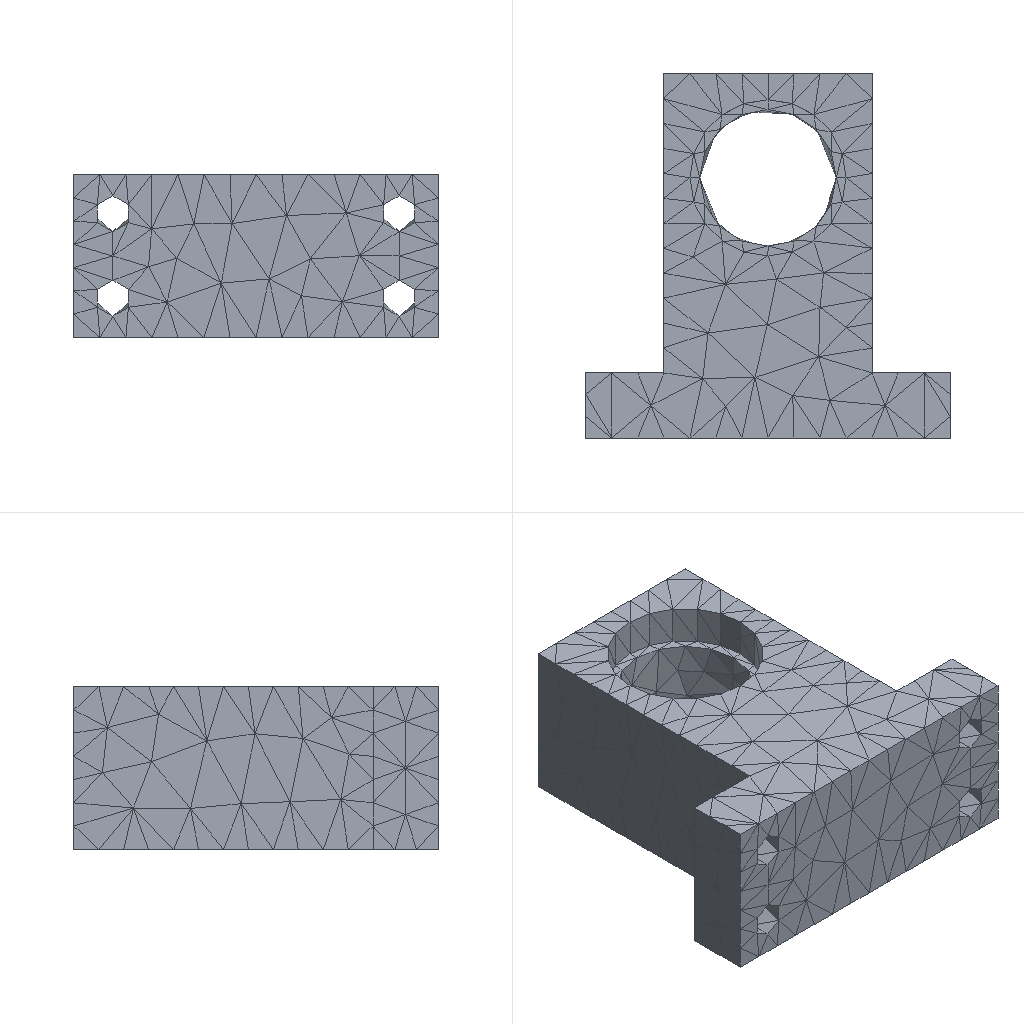Simulation study | ansys mapdl
Set-up summary:
category,name,step,type,value,unit,region
solver,ansys_mapdl
solver,version,,,22.1
units,MPA,,stated
analysis,deck,,transient,transient
load_step,requested,,,1
analysis,nlgeom,,,True
mesh,nodes,,,3282
mesh,elements,,,1777
element_type,ANSYS 187 (type 1),,solid,1667
element_type,ANSYS 154 (type 2),,surface,110
load,load commands in deck,,count,3
bc,support commands in deck,,count,1
named_set,_FIXEDSU,,component
material,1,,in results
check,setup vs results,,match,110 surface effect element(s) are not in the reader's mesh and were not compared
Ansys APDL input file, long lists of numbers shortened:
/batch
/config,noeldb,1     ! force off writing results to database
*get,_wallstrt,active,,time,wall
! ANSYS input file written by Workbench version 2022 R1
! File used for geometry attach: [REDACTED]
/title,___--__ (B5)
! ****** Begin Custom Load Command Snippet ******
/COM, ACT Extensions:
/COM,     LSDYNA, 2021.1
/COM,
! ****** End   Custom Load Command Snippet ******
*DIM,_wb_ProjectScratch_dir,string,248
_wb_ProjectScratch_dir(1) = 'F:\模型汇总\ansys（分析文件汇总)\可动机构（模态，动力学，）\_ProjectScratch\ScrDC28\'
*DIM,_wb_SolverFiles_dir,string,248
_wb_SolverFiles_dir(1) = 'F:\模型汇总\ansys（分析文件汇总)\可动机构（模态，动力学，）\轴承座_files\dp0\SYS-1\MECH\'
*DIM,_wb_userfiles_dir,string,248
_wb_userfiles_dir(1) = 'F:\模型汇总\ansys（分析文件汇总)\可动机构（模态，动力学，）\轴承座_files\user_files\'
/com,--- Data in consistent NMM units. See Solving Units in the help system for more information.
/units,MPA
/nopr
/wb,file,start              !  signify a WB generated input file
/prep7
! Turn off shape checking because checks already performed inside WB mesher.
! See help system for more information.
SHPP,OFF,,NOWARN
/nolist
etcon,set             ! allow ANSYS to choose best KEYOP's for 180x elements, resets any applicable keyopt to MAPDL defaults
/com,*********** Nodes for the whole assembly ***********
nblock,3,,3610
(1i9,3e20.9e3)
        1    -2.200000000E+01    -3.000000000E+01    -9.250000000E+00
! (3281 more lines like these left out)
-1
/wb,elem,start            !  set before creation of elements
/com,*********** Elements for Body 1 "___-FreeParts|____1" ***********
et,1,187
eblock,19,solid,,1667
(19i9)
        1        1        1        1        0        0        0        0       10        0        1      103      563      422      504     1254     2831     1248     1250
! (3333 more lines like these left out)
-1
/wb,elem,end               !  done creating elements
/com,*********** Send User Defined Coordinate System(s) ***********
csys,0
toffst,273.15,  ! Temperature offset from absolute zero
/com,*********** Set Reference Temperature ***********
tref,22.
/wb,mat,start              !  starting to send materials
/com,*********** Send Materials ***********
Temperature = 'TEMP' ! Temperature
MP,DENS,1,7.85e-09,	! tonne mm^-3
MP,ALPX,1,1.2e-05,	! C^-1
MP,C,1,434000000,	! mm^2 s^-2 C^-1
MP,KXX,1,60.5,	! tonne mm s^-3 C^-1
MP,RSVX,1,0.00017,	! ohm mm
MP,EX,1,200000,	! tonne s^-2 mm^-1
MP,NUXY,1,0.3,
MP,MURX,1,10000,
/wb,mat,end                !  done sending materials
!************************* Model Summary ********************
!___-FreeParts|____1,	structural steel,	matid,	1
!************************* End Model Summary ********************
! get the diagonal of the bounding box. Needed later for other things
*get,_xmin,node,,mnloc,x
*get,_ymin,node,,mnloc,y
*get,_zmin,node,,mnloc,z
*get,_xmax,node,,mxloc,x
*get,_ymax,node,,mxloc,y
*get,_zmax,node,,mxloc,z
_ASMDIAG=(_xmax-_xmin)*(_xmax-_xmin)+(_ymax-_ymin)*(_ymax-_ymin)+(_zmax-_zmin)*(_zmax-_zmin)
_ASMDIAG=SQRT(_ASMDIAG)
/wb,contact,start          !  starting to send contact
/wb,contact,end            !  done creating contacts
/golist
/wb,load,start             !  starting to send loads
/com,*********** Fixed Supports ***********
CMBLOCK,_FIXEDSU,NODE,      271
(8i10)
         5         8         9        10        17        20        21        22
! (33 more lines like these left out)
cmsel,s,_FIXEDSU
d,all,all
nsel,all
/com,*********** Define Force Using Surface Effect Elements ***********
local,12,0,0.,0.,0.,0.,0.,0.
csys,0
et,2,154
eblock,10,,,110
(15i9)
     2638        2        2        2       12      182      219      190      190     1658     1690      190     1657
! (109 more lines like these left out)
-1
esel,s,type,,2
keyop,2,2,1                ! Apply load in local coordinate system
keyop,2,7,1                ! Use original area so load is constant in large deformation
esel,all
/gst,on,on
fini
*get,_numnode,node,0,count
*get,_numelem,elem,0,count
*get, _MAXELEMNUM, elem, 0, NUM, MAX
*get, _MAXNODENUM, node, 0, NUM, MAX
*get, _MAXELEMTYPE, etyp, 0, NUM, MAX
*get, _MAXREALCONST, real, 0, NUM, MAX
/go
/wb,load,end               !  done creating loads
/com,--- Number of total nodes = %_numnode%
/com,--- Number of contact elements = 110
/com,--- Number of spring elements = 0
/com,--- Number of bearing elements = 0
/com,--- Number of solid elements = 1667
/com,--- Number of condensed parts = 0
/com,--- Number of total elements = %_numelem%
*get,_wallbsol,active,,time,wall
/com,****************************************************************************
/com,*************************    SOLUTION       ********************************
/com,****************************************************************************
/solu
antype,4                   ! transient analysis
nlgeom,on                  ! Turn on Large Deformation Effects
kbc,1                      ! stepped BC's
_thickRatio=  1     ! Ratio of thick parts in the model
eqsl,pcg,1e-8,,,,,,1
cntr,print,1               ! print out contact info and also make no initial contact an error
dmpoption,emat,no             ! Don't combine emat file for DANSYS
dmpoption,esav,no             ! Don't combine esav file for DANSYS
trnopt,full,,,,,hht        ! HHT time integration method
tintp, mosp			! Choose transient integration settings for moderate speed application
nldiag,cont,iter           ! print out contact info each equilibrium iteration
rescontrol,define,last,last,,dele	   ! Program Controlled
/com,****************************************************
/com,******************* SOLVE FOR LS 1 OF 1 ****************
esel,s,type,,2
nsle
sfe,all,1,pres,1,0.
sfe,all,2,pres,1,0.
sfe,all,3,pres,1,-0.3165
nsel,all
esel,all
/nopr
/gopr
autots,on                   ! User [REDACTED] on automatic time stepping
deltim,20,20,20,OFF
time,20.
timint,on                  ! Turn on time integration effects
outres,erase
outres,all,none
outres,nsol,all,
outres,rsol,all
outres,eangl,all
outres,etmp,all
outres,veng,all
outres,strs,all,
outres,epel,all,
outres,eppl,all,
outres,cont,all,
outres,v,all,
outres,a,all,
! *********** WB SOLVE COMMAND ***********
! check interactive state
*get,ANSINTER_,active,,int
*if,ANSINTER_,ne,0,then
/eof
*endif
solve
/com *************** Write FE CONNECTORS *********
CEWRITE,file,ce,,INTE
/com,****************************************************
/com,*************** FINISHED SOLVE FOR LS 1 *************
*get,_wallasol,active,,time,wall
/nopr
*get,_numnode,node,0,count
*get,_numelem,elem,0,count
*get, _MAXELEMNUM, elem, 0, NUM, MAX
*get, _MAXNODENUM, node, 0, NUM, MAX,,,INTERNAL
*get, _MAXELEMTYPE, etyp, 0, NUM, MAX
*get, _MAXREALCONST, real, 0, NUM, MAX
/gopr
*get,_PCGITER,active,,solu,cgiter
/post1
xmlo,ENCODING,ISO-8859-1
xmlo,parm
/xml,parm,xml
fini
/gopr
*get,_walldone,active,,time,wall
_preptime=(_wallbsol-_wallstrt)*3600
_solvtime=(_wallasol-_wallbsol)*3600
_posttime=(_walldone-_wallasol)*3600
_totaltim=(_walldone-_wallstrt)*3600
*get,_dlbratio,active,0,solu,dlbr
*get,_combtime,active,0,solu,comb
*get,_ssmode,active,0,solu,ssmm
*get,_ndofs,active,0,solu,ndof
*get,_sol_end_time,active,0,set,time
*if,_sol_end_time,eq,20.,then
/fclean				!clean distributed files
*endif
/com,--- Total number of nodes = %_numnode%
/com,--- Total number of elements = %_numelem%
/com,--- Element load balance ratio = %_dlbratio%
/com,--- Time to combine distributed files = %_combtime%
/com,--- Sparse memory mode = %_ssmode%
/com,--- Number of DOF = %_ndofs%
/wb,file,end               ! done with WB generated input
Results summary:
result,analysis,,,static
result,last_loadstep,,,1
result,primary field,,,displacement
result,reaction total,1,FX,-0.0,N
result,reaction total,1,FY,-0.0,N
result,reaction total,1,FZ,500.0,N
result,mass,,,0.000314,"NMM: mm, ton, N, s, mV, mA, degC"